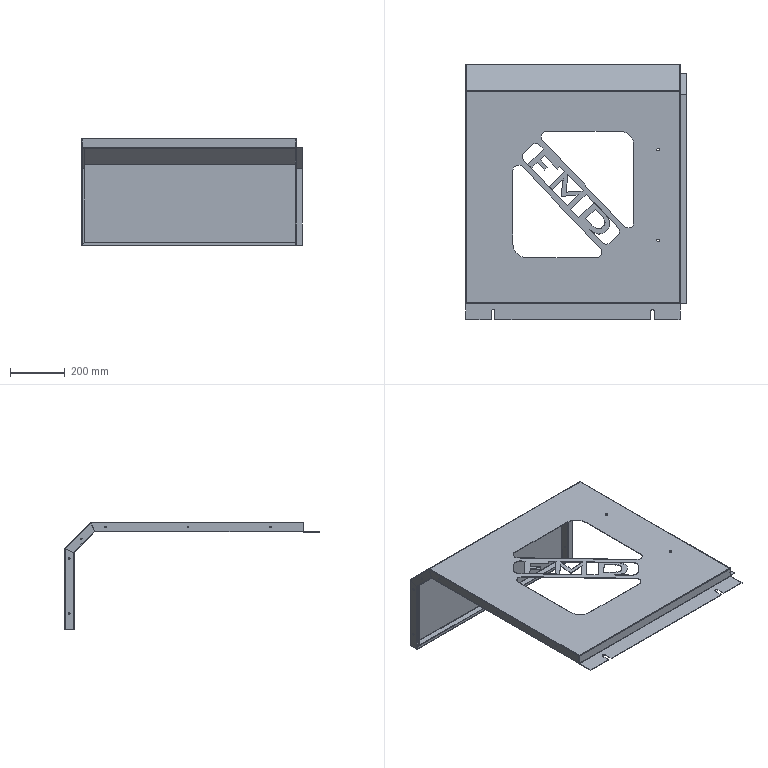Part | STEP file | 520 Sliding Door | 1 solid | 256 faces | box 803 x 928 x 391 mm | volume 1999318 mm3 | plane 139 | cylinder 94 | spline 23 | commonest cylinder face diameters 6 x24 0.2 x18 4.2 x18 0.4 x14 40 x10 9 x4